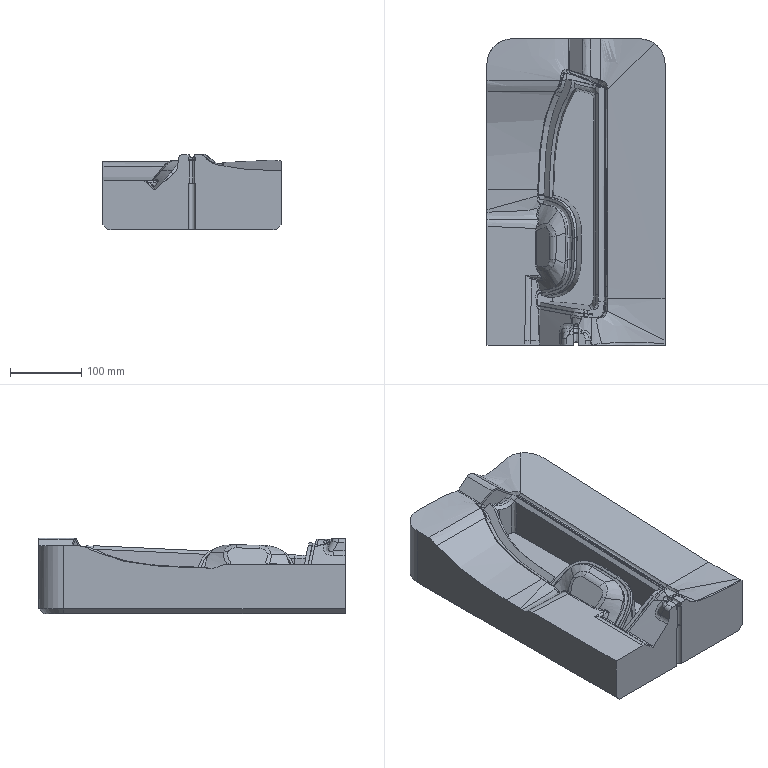Part | STEP file | 4-20.sldasm-Part-378 | 1 solid | 319 faces | box 250.007 x 430 x 106.26 mm | volume 8277486 mm3 | spline 271 | plane 29 | cylinder 14 | cone 4 | torus 1 | commonest cylinder face diameters 12 x3 20 x3 7.95 x2 70 x2 4 x1 6 x1